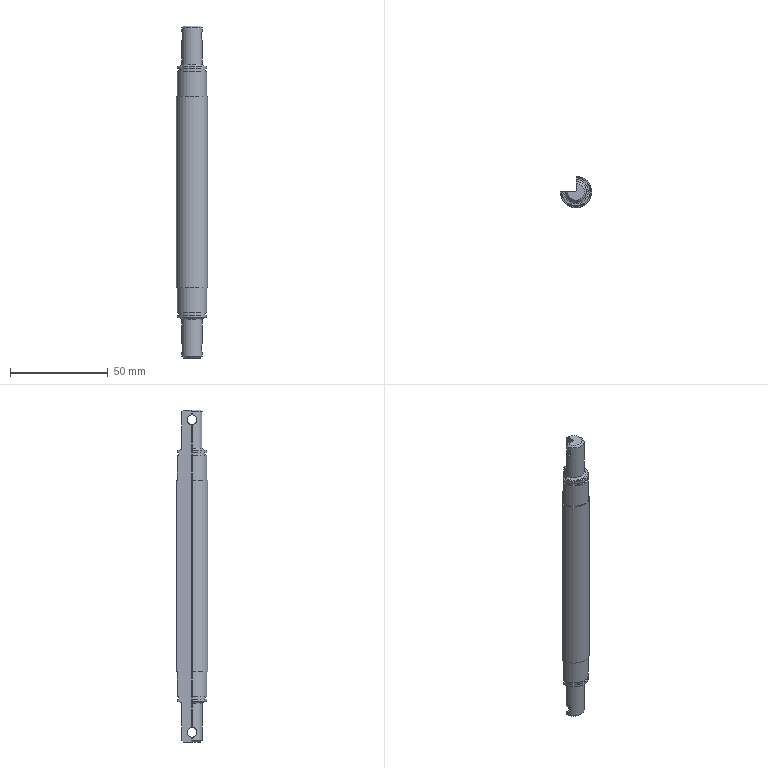Part | STEP file | driven shaft | 1 solid | 69 faces | box 16 x 15.999 x 170 mm | volume 21183 mm3 | cylinder 37 | plane 14 | cone 12 | torus 6 | commonest cylinder face diameters 15 x12 5 x8 10.5 x8 13.8 x6 16 x3